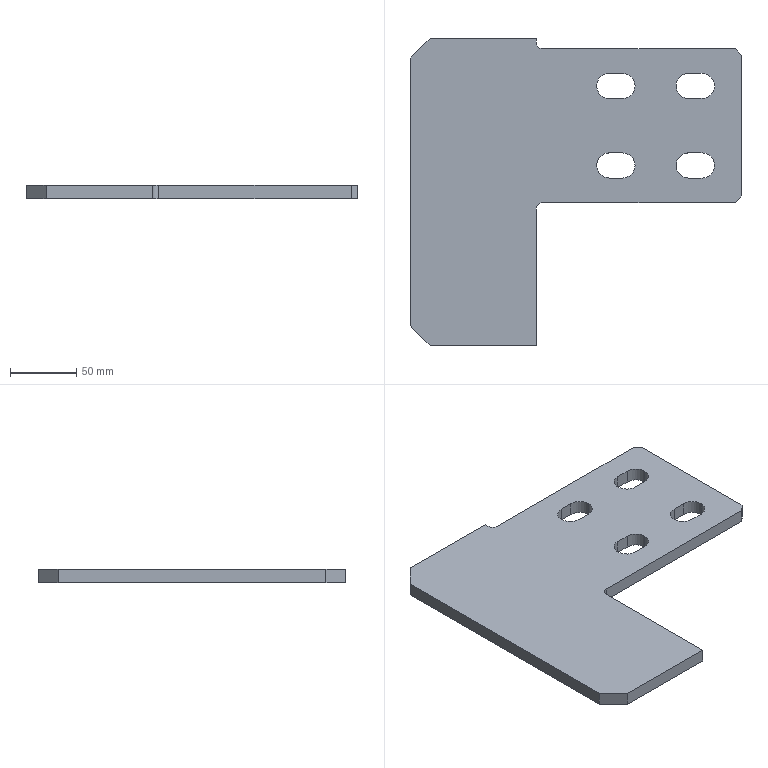Part | STEP file | 筋Plate-250×125-150-30度 | 1 solid | 36 faces | box 250 x 232 x 10 mm | volume 378866 mm3 | plane 22 | cylinder 14 | commonest cylinder face diameters 19 x12 10 x2